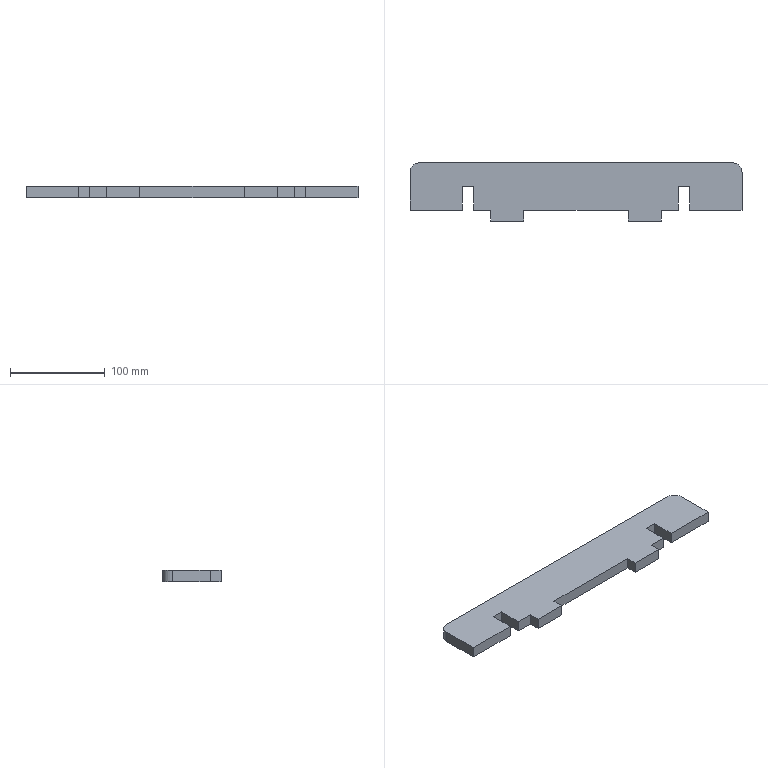Part | SolidWorks | features FlatPattern 1, SMBaseFlange 1, SheetMetal 1 | 1 solid | 24 faces | box 350 x 61.5 x 12 mm | volume 211887 mm3 | plane 22 | cylinder 2 | commonest cylinder face diameters 20 x2
STEP:
#1=CARTESIAN_POINT('',(212.445,-154.972,0.));
#2=VERTEX_POINT('',#1);
#3=CARTESIAN_POINT('',(212.445,-114.972,0.));
#4=VERTEX_POINT('',#3);
#5=CARTESIAN_POINT('',(212.445,-154.972,0.));
#6=DIRECTION('',(0.,1.,0.));
#7=VECTOR('',#6,1000.);
#8=LINE('',#5,#7);
#9=EDGE_CURVE('',#2,#4,#8,.T.);
#10=ORIENTED_EDGE('',*,*,#9,.F.);
#11=CARTESIAN_POINT('',(212.445,-154.972,-12.));
#12=VERTEX_POINT('',#11);
#13=CARTESIAN_POINT('',(212.445,-154.972,-12.));
#14=DIRECTION('',(0.,0.,1.));
#15=VECTOR('',#14,1000.);
#16=LINE('',#13,#15);
#17=EDGE_CURVE('',#12,#2,#16,.T.);
#18=ORIENTED_EDGE('',*,*,#17,.F.);
#19=CARTESIAN_POINT('',(212.445,-114.972,-12.));
#20=VERTEX_POINT('',#19);
#21=CARTESIAN_POINT('',(212.445,-154.972,-12.));
#22=DIRECTION('',(0.,1.,0.));
#23=VECTOR('',#22,1000.);
#24=LINE('',#21,#23);
#25=EDGE_CURVE('',#12,#20,#24,.T.);
#26=ORIENTED_EDGE('',*,*,#25,.T.);
#27=CARTESIAN_POINT('',(212.445,-114.972,-12.));
#28=DIRECTION('',(0.,0.,1.));
#29=VECTOR('',#28,1000.);
#30=LINE('',#27,#29);
#31=EDGE_CURVE('',#20,#4,#30,.T.);
#32=ORIENTED_EDGE('',*,*,#31,.T.);
#33=EDGE_LOOP('',(#10,#18,#26,#32));
#34=FACE_OUTER_BOUND('',#33,.T.);
#35=CARTESIAN_POINT('',(212.445,-154.972,-12.));
#36=DIRECTION('',(1.,0.,0.));
#37=DIRECTION('',(0.,0.,-1.));
#38=AXIS2_PLACEMENT_3D('',#35,#36,#37);
#39=PLANE('',#38);
#40=ADVANCED_FACE('',(#34),#39,.T.);
#41=CARTESIAN_POINT('',(157.445,-154.972,0.));
#42=VERTEX_POINT('',#41);
#43=CARTESIAN_POINT('',(212.445,-154.972,0.));
#44=DIRECTION('',(1.,0.,0.));
#45=VECTOR('',#44,1000.);
#46=LINE('',#43,#45);
#47=EDGE_CURVE('',#42,#2,#46,.T.);
#48=ORIENTED_EDGE('',*,*,#47,.F.);
#49=CARTESIAN_POINT('',(157.445,-154.972,-12.));
#50=VERTEX_POINT('',#49);
#51=CARTESIAN_POINT('',(157.445,-154.972,-12.));
#52=DIRECTION('',(0.,0.,1.));
#53=VECTOR('',#52,1000.);
#54=LINE('',#51,#53);
#55=EDGE_CURVE('',#50,#42,#54,.T.);
#56=ORIENTED_EDGE('',*,*,#55,.F.);
#57=CARTESIAN_POINT('',(212.445,-154.972,-12.));
#58=DIRECTION('',(1.,0.,0.));
#59=VECTOR('',#58,1000.);
#60=LINE('',#57,#59);
#61=EDGE_CURVE('',#50,#12,#60,.T.);
#62=ORIENTED_EDGE('',*,*,#61,.T.);
#63=ORIENTED_EDGE('',*,*,#17,.T.);
#64=EDGE_LOOP('',(#48,#56,#62,#63));
#65=FACE_OUTER_BOUND('',#64,.T.);
#66=CARTESIAN_POINT('',(212.445,-154.972,-12.));
#67=DIRECTION('',(0.,-1.,0.));
#68=DIRECTION('',(1.,0.,0.));
#69=AXIS2_PLACEMENT_3D('',#66,#67,#68);
#70=PLANE('',#69);
#71=ADVANCED_FACE('',(#65),#70,.T.);
#72=CARTESIAN_POINT('',(157.445,-129.772,0.));
#73=VERTEX_POINT('',#72);
#74=CARTESIAN_POINT('',(157.445,-129.772,0.));
#75=DIRECTION('',(0.,-1.,0.));
#76=VECTOR('',#75,1000.);
#77=LINE('',#74,#76);
#78=EDGE_CURVE('',#73,#42,#77,.T.);
#79=ORIENTED_EDGE('',*,*,#78,.F.);
#80=CARTESIAN_POINT('',(157.445,-129.772,-12.));
#81=VERTEX_POINT('',#80);
#82=CARTESIAN_POINT('',(157.445,-129.772,-12.));
#83=DIRECTION('',(0.,0.,1.));
#84=VECTOR('',#83,1000.);
#85=LINE('',#82,#84);
#86=EDGE_CURVE('',#81,#73,#85,.T.);
#87=ORIENTED_EDGE('',*,*,#86,.F.);
#88=CARTESIAN_POINT('',(157.445,-129.772,-12.));
#89=DIRECTION('',(0.,-1.,0.));
#90=VECTOR('',#89,1000.);
#91=LINE('',#88,#90);
#92=EDGE_CURVE('',#81,#50,#91,.T.);
#93=ORIENTED_EDGE('',*,*,#92,.T.);
#94=ORIENTED_EDGE('',*,*,#55,.T.);
#95=EDGE_LOOP('',(#79,#87,#93,#94));
#96=FACE_OUTER_BOUND('',#95,.T.);
#97=CARTESIAN_POINT('',(157.445,-129.772,-12.));
#98=DIRECTION('',(-1.,0.,0.));
#99=DIRECTION('',(0.,0.,1.));
#100=AXIS2_PLACEMENT_3D('',#97,#98,#99);
#101=PLANE('',#100);
#102=ADVANCED_FACE('',(#96),#101,.T.);
#103=CARTESIAN_POINT('',(145.445,-129.772,0.));
#104=VERTEX_POINT('',#103);
#105=CARTESIAN_POINT('',(145.445,-129.772,0.));
#106=DIRECTION('',(1.,0.,0.));
#107=VECTOR('',#106,1000.);
#108=LINE('',#105,#107);
#109=EDGE_CURVE('',#104,#73,#108,.T.);
#110=ORIENTED_EDGE('',*,*,#109,.F.);
#111=CARTESIAN_POINT('',(145.445,-129.772,-12.));
#112=VERTEX_POINT('',#111);
#113=CARTESIAN_POINT('',(145.445,-129.772,-12.));
#114=DIRECTION('',(0.,0.,1.));
#115=VECTOR('',#114,1000.);
#116=LINE('',#113,#115);
#117=EDGE_CURVE('',#112,#104,#116,.T.);
#118=ORIENTED_EDGE('',*,*,#117,.F.);
#119=CARTESIAN_POINT('',(145.445,-129.772,-12.));
#120=DIRECTION('',(1.,0.,0.));
#121=VECTOR('',#120,1000.);
#122=LINE('',#119,#121);
#123=EDGE_CURVE('',#112,#81,#122,.T.);
#124=ORIENTED_EDGE('',*,*,#123,.T.);
#125=ORIENTED_EDGE('',*,*,#86,.T.);
#126=EDGE_LOOP('',(#110,#118,#124,#125));
#127=FACE_OUTER_BOUND('',#126,.T.);
#128=CARTESIAN_POINT('',(145.445,-129.772,-12.));
#129=DIRECTION('',(0.,-1.,0.));
#130=DIRECTION('',(0.,0.,-1.));
#131=AXIS2_PLACEMENT_3D('',#128,#129,#130);
#132=PLANE('',#131);
#133=ADVANCED_FACE('',(#127),#132,.T.);
#134=CARTESIAN_POINT('',(145.445,-154.972,0.));
#135=VERTEX_POINT('',#134);
#136=CARTESIAN_POINT('',(145.445,-154.972,0.));
#137=DIRECTION('',(0.,1.,0.));
#138=VECTOR('',#137,1000.);
#139=LINE('',#136,#138);
#140=EDGE_CURVE('',#135,#104,#139,.T.);
#141=ORIENTED_EDGE('',*,*,#140,.F.);
#142=CARTESIAN_POINT('',(145.445,-154.972,-12.));
#143=VERTEX_POINT('',#142);
#144=CARTESIAN_POINT('',(145.445,-154.972,-12.));
#145=DIRECTION('',(0.,0.,1.));
#146=VECTOR('',#145,1000.);
#147=LINE('',#144,#146);
#148=EDGE_CURVE('',#143,#135,#147,.T.);
#149=ORIENTED_EDGE('',*,*,#148,.F.);
#150=CARTESIAN_POINT('',(145.445,-154.972,-12.));
#151=DIRECTION('',(0.,1.,0.));
#152=VECTOR('',#151,1000.);
#153=LINE('',#150,#152);
#154=EDGE_CURVE('',#143,#112,#153,.T.);
#155=ORIENTED_EDGE('',*,*,#154,.T.);
#156=ORIENTED_EDGE('',*,*,#117,.T.);
#157=EDGE_LOOP('',(#141,#149,#155,#156));
#158=FACE_OUTER_BOUND('',#157,.T.);
#159=CARTESIAN_POINT('',(145.445,-154.972,-12.));
#160=DIRECTION('',(1.,0.,0.));
#161=DIRECTION('',(0.,0.,-1.));
#162=AXIS2_PLACEMENT_3D('',#159,#160,#161);
#163=PLANE('',#162);
#164=ADVANCED_FACE('',(#158),#163,.T.);
#165=CARTESIAN_POINT('',(127.445,-154.972,0.));
#166=VERTEX_POINT('',#165);
#167=CARTESIAN_POINT('',(145.445,-154.972,0.));
#168=DIRECTION('',(1.,0.,0.));
#169=VECTOR('',#168,1000.);
#170=LINE('',#167,#169);
#171=EDGE_CURVE('',#166,#135,#170,.T.);
#172=ORIENTED_EDGE('',*,*,#171,.F.);
#173=CARTESIAN_POINT('',(127.445,-154.972,-12.));
#174=VERTEX_POINT('',#173);
#175=CARTESIAN_POINT('',(127.445,-154.972,-12.));
#176=DIRECTION('',(0.,0.,1.));
#177=VECTOR('',#176,1000.);
#178=LINE('',#175,#177);
#179=EDGE_CURVE('',#174,#166,#178,.T.);
#180=ORIENTED_EDGE('',*,*,#179,.F.);
#181=CARTESIAN_POINT('',(145.445,-154.972,-12.));
#182=DIRECTION('',(1.,0.,0.));
#183=VECTOR('',#182,1000.);
#184=LINE('',#181,#183);
#185=EDGE_CURVE('',#174,#143,#184,.T.);
#186=ORIENTED_EDGE('',*,*,#185,.T.);
#187=ORIENTED_EDGE('',*,*,#148,.T.);
#188=EDGE_LOOP('',(#172,#180,#186,#187));
#189=FACE_OUTER_BOUND('',#188,.T.);
#190=CARTESIAN_POINT('',(145.445,-154.972,-12.));
#191=DIRECTION('',(0.,-1.,0.));
#192=DIRECTION('',(1.,0.,0.));
#193=AXIS2_PLACEMENT_3D('',#190,#191,#192);
#194=PLANE('',#193);
#195=ADVANCED_FACE('',(#189),#194,.T.);
#196=CARTESIAN_POINT('',(127.445,-166.472,0.));
#197=VERTEX_POINT('',#196);
#198=CARTESIAN_POINT('',(127.445,-154.972,0.));
#199=DIRECTION('',(0.,1.,0.));
#200=VECTOR('',#199,1000.);
#201=LINE('',#198,#200);
#202=EDGE_CURVE('',#197,#166,#201,.T.);
#203=ORIENTED_EDGE('',*,*,#202,.F.);
#204=CARTESIAN_POINT('',(127.445,-166.472,-12.));
#205=VERTEX_POINT('',#204);
#206=CARTESIAN_POINT('',(127.445,-166.472,-12.));
#207=DIRECTION('',(0.,0.,1.));
#208=VECTOR('',#207,1000.);
#209=LINE('',#206,#208);
#210=EDGE_CURVE('',#205,#197,#209,.T.);
#211=ORIENTED_EDGE('',*,*,#210,.F.);
#212=CARTESIAN_POINT('',(127.445,-154.972,-12.));
#213=DIRECTION('',(0.,1.,0.));
#214=VECTOR('',#213,1000.);
#215=LINE('',#212,#214);
#216=EDGE_CURVE('',#205,#174,#215,.T.);
#217=ORIENTED_EDGE('',*,*,#216,.T.);
#218=ORIENTED_EDGE('',*,*,#179,.T.);
#219=EDGE_LOOP('',(#203,#211,#217,#218));
#220=FACE_OUTER_BOUND('',#219,.T.);
#221=CARTESIAN_POINT('',(127.445,-154.972,-12.));
#222=DIRECTION('',(1.,0.,0.));
#223=DIRECTION('',(0.,1.,0.));
#224=AXIS2_PLACEMENT_3D('',#221,#222,#223);
#225=PLANE('',#224);
#226=ADVANCED_FACE('',(#220),#225,.T.);
#227=CARTESIAN_POINT('',(92.445,-166.472,0.));
#228=VERTEX_POINT('',#227);
#229=CARTESIAN_POINT('',(127.445,-166.472,0.));
#230=DIRECTION('',(1.,0.,0.));
#231=VECTOR('',#230,1000.);
#232=LINE('',#229,#231);
#233=EDGE_CURVE('',#228,#197,#232,.T.);
#234=ORIENTED_EDGE('',*,*,#233,.F.);
#235=CARTESIAN_POINT('',(92.445,-166.472,-12.));
#236=VERTEX_POINT('',#235);
#237=CARTESIAN_POINT('',(92.445,-166.472,-12.));
#238=DIRECTION('',(0.,0.,1.));
#239=VECTOR('',#238,1000.);
#240=LINE('',#237,#239);
#241=EDGE_CURVE('',#236,#228,#240,.T.);
#242=ORIENTED_EDGE('',*,*,#241,.F.);
#243=CARTESIAN_POINT('',(127.445,-166.472,-12.));
#244=DIRECTION('',(1.,0.,0.));
#245=VECTOR('',#244,1000.);
#246=LINE('',#243,#245);
#247=EDGE_CURVE('',#236,#205,#246,.T.);
#248=ORIENTED_EDGE('',*,*,#247,.T.);
#249=ORIENTED_EDGE('',*,*,#210,.T.);
#250=EDGE_LOOP('',(#234,#242,#248,#249));
#251=FACE_OUTER_BOUND('',#250,.T.);
#252=CARTESIAN_POINT('',(127.445,-166.472,-12.));
#253=DIRECTION('',(0.,-1.,0.));
#254=DIRECTION('',(0.,0.,-1.));
#255=AXIS2_PLACEMENT_3D('',#252,#253,#254);
#256=PLANE('',#255);
#257=ADVANCED_FACE('',(#251),#256,.T.);
#258=CARTESIAN_POINT('',(92.445,-154.972,0.));
#259=VERTEX_POINT('',#258);
#260=CARTESIAN_POINT('',(92.445,-166.472,0.));
#261=DIRECTION('',(0.,-1.,0.));
#262=VECTOR('',#261,1000.);
#263=LINE('',#260,#262);
#264=EDGE_CURVE('',#259,#228,#263,.T.);
#265=ORIENTED_EDGE('',*,*,#264,.F.);
#266=CARTESIAN_POINT('',(92.445,-154.972,-12.));
#267=VERTEX_POINT('',#266);
#268=CARTESIAN_POINT('',(92.445,-154.972,-12.));
#269=DIRECTION('',(0.,0.,1.));
#270=VECTOR('',#269,1000.);
#271=LINE('',#268,#270);
#272=EDGE_CURVE('',#267,#259,#271,.T.);
#273=ORIENTED_EDGE('',*,*,#272,.F.);
#274=CARTESIAN_POINT('',(92.445,-166.472,-12.));
#275=DIRECTION('',(0.,-1.,0.));
#276=VECTOR('',#275,1000.);
#277=LINE('',#274,#276);
#278=EDGE_CURVE('',#267,#236,#277,.T.);
#279=ORIENTED_EDGE('',*,*,#278,.T.);
#280=ORIENTED_EDGE('',*,*,#241,.T.);
#281=EDGE_LOOP('',(#265,#273,#279,#280));
#282=FACE_OUTER_BOUND('',#281,.T.);
#283=CARTESIAN_POINT('',(92.445,-166.472,-12.));
#284=DIRECTION('',(-1.,0.,0.));
#285=DIRECTION('',(0.,0.,1.));
#286=AXIS2_PLACEMENT_3D('',#283,#284,#285);
#287=PLANE('',#286);
#288=ADVANCED_FACE('',(#282),#287,.T.);
#289=CARTESIAN_POINT('',(-17.555,-154.972,0.));
#290=VERTEX_POINT('',#289);
#291=CARTESIAN_POINT('',(92.445,-154.972,0.));
#292=DIRECTION('',(1.,0.,0.));
#293=VECTOR('',#292,1000.);
#294=LINE('',#291,#293);
#295=EDGE_CURVE('',#290,#259,#294,.T.);
#296=ORIENTED_EDGE('',*,*,#295,.F.);
#297=CARTESIAN_POINT('',(-17.555,-154.972,-12.));
#298=VERTEX_POINT('',#297);
#299=CARTESIAN_POINT('',(-17.555,-154.972,-12.));
#300=DIRECTION('',(0.,0.,1.));
#301=VECTOR('',#300,1000.);
#302=LINE('',#299,#301);
#303=EDGE_CURVE('',#298,#290,#302,.T.);
#304=ORIENTED_EDGE('',*,*,#303,.F.);
#305=CARTESIAN_POINT('',(92.445,-154.972,-12.));
#306=DIRECTION('',(1.,0.,0.));
#307=VECTOR('',#306,1000.);
#308=LINE('',#305,#307);
#309=EDGE_CURVE('',#298,#267,#308,.T.);
#310=ORIENTED_EDGE('',*,*,#309,.T.);
#311=ORIENTED_EDGE('',*,*,#272,.T.);
#312=EDGE_LOOP('',(#296,#304,#310,#311));
#313=FACE_OUTER_BOUND('',#312,.T.);
#314=CARTESIAN_POINT('',(92.445,-154.972,-12.));
#315=DIRECTION('',(0.,-1.,0.));
#316=DIRECTION('',(0.,0.,-1.));
#317=AXIS2_PLACEMENT_3D('',#314,#315,#316);
#318=PLANE('',#317);
#319=ADVANCED_FACE('',(#313),#318,.T.);
#320=CARTESIAN_POINT('',(-17.555,-166.472,0.));
#321=VERTEX_POINT('',#320);
#322=CARTESIAN_POINT('',(-17.555,-166.472,0.));
#323=DIRECTION('',(0.,1.,0.));
#324=VECTOR('',#323,1000.);
#325=LINE('',#322,#324);
#326=EDGE_CURVE('',#321,#290,#325,.T.);
#327=ORIENTED_EDGE('',*,*,#326,.F.);
#328=CARTESIAN_POINT('',(-17.555,-166.472,-12.));
#329=VERTEX_POINT('',#328);
#330=CARTESIAN_POINT('',(-17.555,-166.472,-12.));
#331=DIRECTION('',(0.,0.,1.));
#332=VECTOR('',#331,1000.);
#333=LINE('',#330,#332);
#334=EDGE_CURVE('',#329,#321,#333,.T.);
#335=ORIENTED_EDGE('',*,*,#334,.F.);
#336=CARTESIAN_POINT('',(-17.555,-166.472,-12.));
#337=DIRECTION('',(0.,1.,0.));
#338=VECTOR('',#337,1000.);
#339=LINE('',#336,#338);
#340=EDGE_CURVE('',#329,#298,#339,.T.);
#341=ORIENTED_EDGE('',*,*,#340,.T.);
#342=ORIENTED_EDGE('',*,*,#303,.T.);
#343=EDGE_LOOP('',(#327,#335,#341,#342));
#344=FACE_OUTER_BOUND('',#343,.T.);
#345=CARTESIAN_POINT('',(-17.555,-166.472,-12.));
#346=DIRECTION('',(1.,0.,0.));
#347=DIRECTION('',(0.,0.,-1.));
#348=AXIS2_PLACEMENT_3D('',#345,#346,#347);
#349=PLANE('',#348);
#350=ADVANCED_FACE('',(#344),#349,.T.);
#351=CARTESIAN_POINT('',(-52.555,-166.472,0.));
#352=VERTEX_POINT('',#351);
#353=CARTESIAN_POINT('',(-52.555,-166.472,0.));
#354=DIRECTION('',(1.,0.,0.));
#355=VECTOR('',#354,1000.);
#356=LINE('',#353,#355);
#357=EDGE_CURVE('',#352,#321,#356,.T.);
#358=ORIENTED_EDGE('',*,*,#357,.F.);
#359=CARTESIAN_POINT('',(-52.555,-166.472,-12.));
#360=VERTEX_POINT('',#359);
#361=CARTESIAN_POINT('',(-52.555,-166.472,-12.));
#362=DIRECTION('',(0.,0.,1.));
#363=VECTOR('',#362,1000.);
#364=LINE('',#361,#363);
#365=EDGE_CURVE('',#360,#352,#364,.T.);
#366=ORIENTED_EDGE('',*,*,#365,.F.);
#367=CARTESIAN_POINT('',(-52.555,-166.472,-12.));
#368=DIRECTION('',(1.,0.,0.));
#369=VECTOR('',#368,1000.);
#370=LINE('',#367,#369);
#371=EDGE_CURVE('',#360,#329,#370,.T.);
#372=ORIENTED_EDGE('',*,*,#371,.T.);
#373=ORIENTED_EDGE('',*,*,#334,.T.);
#374=EDGE_LOOP('',(#358,#366,#372,#373));
#375=FACE_OUTER_BOUND('',#374,.T.);
#376=CARTESIAN_POINT('',(-52.555,-166.472,-12.));
#377=DIRECTION('',(0.,-1.,0.));
#378=DIRECTION('',(0.,0.,-1.));
#379=AXIS2_PLACEMENT_3D('',#376,#377,#378);
#380=PLANE('',#379);
#381=ADVANCED_FACE('',(#375),#380,.T.);
#382=CARTESIAN_POINT('',(-52.555,-154.972,0.));
#383=VERTEX_POINT('',#382);
#384=CARTESIAN_POINT('',(-52.555,-154.972,0.));
#385=DIRECTION('',(0.,-1.,0.));
#386=VECTOR('',#385,1000.);
#387=LINE('',#384,#386);
#388=EDGE_CURVE('',#383,#352,#387,.T.);
#389=ORIENTED_EDGE('',*,*,#388,.F.);
#390=CARTESIAN_POINT('',(-52.555,-154.972,-12.));
#391=VERTEX_POINT('',#390);
#392=CARTESIAN_POINT('',(-52.555,-154.972,-12.));
#393=DIRECTION('',(0.,0.,1.));
#394=VECTOR('',#393,1000.);
#395=LINE('',#392,#394);
#396=EDGE_CURVE('',#391,#383,#395,.T.);
#397=ORIENTED_EDGE('',*,*,#396,.F.);
#398=CARTESIAN_POINT('',(-52.555,-154.972,-12.));
#399=DIRECTION('',(0.,-1.,0.));
#400=VECTOR('',#399,1000.);
#401=LINE('',#398,#400);
#402=EDGE_CURVE('',#391,#360,#401,.T.);
#403=ORIENTED_EDGE('',*,*,#402,.T.);
#404=ORIENTED_EDGE('',*,*,#365,.T.);
#405=EDGE_LOOP('',(#389,#397,#403,#404));
#406=FACE_OUTER_BOUND('',#405,.T.);
#407=CARTESIAN_POINT('',(-52.555,-154.972,-12.));
#408=DIRECTION('',(-1.,0.,0.));
#409=DIRECTION('',(0.,-1.,0.));
#410=AXIS2_PLACEMENT_3D('',#407,#408,#409);
#411=PLANE('',#410);
#412=ADVANCED_FACE('',(#406),#411,.T.);
#413=CARTESIAN_POINT('',(-70.555,-154.972,0.));
#414=VERTEX_POINT('',#413);
#415=CARTESIAN_POINT('',(-52.555,-154.972,0.));
#416=DIRECTION('',(1.,0.,0.));
#417=VECTOR('',#416,1000.);
#418=LINE('',#415,#417);
#419=EDGE_CURVE('',#414,#383,#418,.T.);
#420=ORIENTED_EDGE('',*,*,#419,.F.);
#421=CARTESIAN_POINT('',(-70.555,-154.972,-12.));
#422=VERTEX_POINT('',#421);
#423=CARTESIAN_POINT('',(-70.555,-154.972,-12.));
#424=DIRECTION('',(0.,0.,1.));
#425=VECTOR('',#424,1000.);
#426=LINE('',#423,#425);
#427=EDGE_CURVE('',#422,#414,#426,.T.);
#428=ORIENTED_EDGE('',*,*,#427,.F.);
#429=CARTESIAN_POINT('',(-52.555,-154.972,-12.));
#430=DIRECTION('',(1.,0.,0.));
#431=VECTOR('',#430,1000.);
#432=LINE('',#429,#431);
#433=EDGE_CURVE('',#422,#391,#432,.T.);
#434=ORIENTED_EDGE('',*,*,#433,.T.);
#435=ORIENTED_EDGE('',*,*,#396,.T.);
#436=EDGE_LOOP('',(#420,#428,#434,#435));
#437=FACE_OUTER_BOUND('',#436,.T.);
#438=CARTESIAN_POINT('',(-52.555,-154.972,-12.));
#439=DIRECTION('',(0.,-1.,0.));
#440=DIRECTION('',(1.,0.,0.));
#441=AXIS2_PLACEMENT_3D('',#438,#439,#440);
#442=PLANE('',#441);
#443=ADVANCED_FACE('',(#437),#442,.T.);
#444=CARTESIAN_POINT('',(-70.555,-129.772,0.));
#445=VERTEX_POINT('',#444);
#446=CARTESIAN_POINT('',(-70.555,-129.772,0.));
#447=DIRECTION('',(0.,-1.,0.));
#448=VECTOR('',#447,1000.);
#449=LINE('',#446,#448);
#450=EDGE_CURVE('',#445,#414,#449,.T.);
#451=ORIENTED_EDGE('',*,*,#450,.F.);
#452=CARTESIAN_POINT('',(-70.555,-129.772,-12.));
#453=VERTEX_POINT('',#452);
#454=CARTESIAN_POINT('',(-70.555,-129.772,-12.));
#455=DIRECTION('',(0.,0.,1.));
#456=VECTOR('',#455,1000.);
#457=LINE('',#454,#456);
#458=EDGE_CURVE('',#453,#445,#457,.T.);
#459=ORIENTED_EDGE('',*,*,#458,.F.);
#460=CARTESIAN_POINT('',(-70.555,-129.772,-12.));
#461=DIRECTION('',(0.,-1.,0.));
#462=VECTOR('',#461,1000.);
#463=LINE('',#460,#462);
#464=EDGE_CURVE('',#453,#422,#463,.T.);
#465=ORIENTED_EDGE('',*,*,#464,.T.);
#466=ORIENTED_EDGE('',*,*,#427,.T.);
#467=EDGE_LOOP('',(#451,#459,#465,#466));
#468=FACE_OUTER_BOUND('',#467,.T.);
#469=CARTESIAN_POINT('',(-70.555,-129.772,-12.));
#470=DIRECTION('',(-1.,0.,0.));
#471=DIRECTION('',(0.,0.,1.));
#472=AXIS2_PLACEMENT_3D('',#469,#470,#471);
#473=PLANE('',#472);
#474=ADVANCED_FACE('',(#468),#473,.T.);
#475=CARTESIAN_POINT('',(-82.555,-129.772,0.));
#476=VERTEX_POINT('',#475);
#477=CARTESIAN_POINT('',(-82.555,-129.772,0.));
#478=DIRECTION('',(1.,0.,0.));
#479=VECTOR('',#478,1000.);
#480=LINE('',#477,#479);
#481=EDGE_CURVE('',#476,#445,#480,.T.);
#482=ORIENTED_EDGE('',*,*,#481,.F.);
#483=CARTESIAN_POINT('',(-82.555,-129.772,-12.));
#484=VERTEX_POINT('',#483);
#485=CARTESIAN_POINT('',(-82.555,-129.772,-12.));
#486=DIRECTION('',(0.,0.,1.));
#487=VECTOR('',#486,1000.);
#488=LINE('',#485,#487);
#489=EDGE_CURVE('',#484,#476,#488,.T.);
#490=ORIENTED_EDGE('',*,*,#489,.F.);
#491=CARTESIAN_POINT('',(-82.555,-129.772,-12.));
#492=DIRECTION('',(1.,0.,0.));
#493=VECTOR('',#492,1000.);
#494=LINE('',#491,#493);
#495=EDGE_CURVE('',#484,#453,#494,.T.);
#496=ORIENTED_EDGE('',*,*,#495,.T.);
#497=ORIENTED_EDGE('',*,*,#458,.T.);
#498=EDGE_LOOP('',(#482,#490,#496,#497));
#499=FACE_OUTER_BOUND('',#498,.T.);
#500=CARTESIAN_POINT('',(-82.555,-129.772,-12.));
#501=DIRECTION('',(0.,-1.,0.));
#502=DIRECTION('',(0.,0.,-1.));
#503=AXIS2_PLACEMENT_3D('',#500,#501,#502);
#504=PLANE('',#503);
#505=ADVANCED_FACE('',(#499),#504,.T.);
#506=CARTESIAN_POINT('',(-82.555,-154.972,0.));
#507=VERTEX_POINT('',#506);
#508=CARTESIAN_POINT('',(-82.555,-154.972,0.));
#509=DIRECTION('',(0.,1.,0.));
#510=VECTOR('',#509,1000.);
#511=LINE('',#508,#510);
#512=EDGE_CURVE('',#507,#476,#511,.T.);
#513=ORIENTED_EDGE('',*,*,#512,.F.);
#514=CARTESIAN_POINT('',(-82.555,-154.972,-12.));
#515=VERTEX_POINT('',#514);
#516=CARTESIAN_POINT('',(-82.555,-154.972,-12.));
#517=DIRECTION('',(0.,0.,1.));
#518=VECTOR('',#517,1000.);
#519=LINE('',#516,#518);
#520=EDGE_CURVE('',#515,#507,#519,.T.);
#521=ORIENTED_EDGE('',*,*,#520,.F.);
#522=CARTESIAN_POINT('',(-82.555,-154.972,-12.));
#523=DIRECTION('',(0.,1.,0.));
#524=VECTOR('',#523,1000.);
#525=LINE('',#522,#524);
#526=EDGE_CURVE('',#515,#484,#525,.T.);
#527=ORIENTED_EDGE('',*,*,#526,.T.);
#528=ORIENTED_EDGE('',*,*,#489,.T.);
#529=EDGE_LOOP('',(#513,#521,#527,#528));
#530=FACE_OUTER_BOUND('',#529,.T.);
#531=CARTESIAN_POINT('',(-82.555,-154.972,-12.));
#532=DIRECTION('',(1.,0.,0.));
#533=DIRECTION('',(0.,0.,-1.));
#534=AXIS2_PLACEMENT_3D('',#531,#532,#533);
#535=PLANE('',#534);
#536=ADVANCED_FACE('',(#530),#535,.T.);
#537=CARTESIAN_POINT('',(-137.555,-154.972,0.));
#538=VERTEX_POINT('',#537);
#539=CARTESIAN_POINT('',(-82.555,-154.972,0.));
#540=DIRECTION('',(1.,0.,0.));
#541=VECTOR('',#540,1000.);
#542=LINE('',#539,#541);
#543=EDGE_CURVE('',#538,#507,#542,.T.);
#544=ORIENTED_EDGE('',*,*,#543,.F.);
#545=CARTESIAN_POINT('',(-137.555,-154.972,-12.));
#546=VERTEX_POINT('',#545);
#547=CARTESIAN_POINT('',(-137.555,-154.972,-12.));
#548=DIRECTION('',(0.,0.,1.));
#549=VECTOR('',#548,1000.);
#550=LINE('',#547,#549);
#551=EDGE_CURVE('',#546,#538,#550,.T.);
#552=ORIENTED_EDGE('',*,*,#551,.F.);
#553=CARTESIAN_POINT('',(-82.555,-154.972,-12.));
#554=DIRECTION('',(1.,0.,0.));
#555=VECTOR('',#554,1000.);
#556=LINE('',#553,#555);
#557=EDGE_CURVE('',#546,#515,#556,.T.);
#558=ORIENTED_EDGE('',*,*,#557,.T.);
#559=ORIENTED_EDGE('',*,*,#520,.T.);
#560=EDGE_LOOP('',(#544,#552,#558,#559));
#561=FACE_OUTER_BOUND('',#560,.T.);
#562=CARTESIAN_POINT('',(-82.555,-154.972,-12.));
#563=DIRECTION('',(0.,-1.,0.));
#564=DIRECTION('',(1.,0.,0.));
#565=AXIS2_PLACEMENT_3D('',#562,#563,#564);
#566=PLANE('',#565);
#567=ADVANCED_FACE('',(#561),#566,.T.);
#568=CARTESIAN_POINT('',(-137.555,-114.972,0.));
#569=VERTEX_POINT('',#568);
#570=CARTESIAN_POINT('',(-137.555,-154.972,0.));
#571=DIRECTION('',(0.,-1.,0.));
#572=VECTOR('',#571,1000.);
#573=LINE('',#570,#572);
#574=EDGE_CURVE('',#569,#538,#573,.T.);
#575=ORIENTED_EDGE('',*,*,#574,.F.);
#576=CARTESIAN_POINT('',(-137.555,-114.972,-12.));
#577=VERTEX_POINT('',#576);
#578=CARTESIAN_POINT('',(-137.555,-114.972,-12.));
#579=DIRECTION('',(0.,0.,1.));
#580=VECTOR('',#579,1000.);
#581=LINE('',#578,#580);
#582=EDGE_CURVE('',#577,#569,#581,.T.);
#583=ORIENTED_EDGE('',*,*,#582,.F.);
#584=CARTESIAN_POINT('',(-137.555,-154.972,-12.));
#585=DIRECTION('',(0.,-1.,0.));
#586=VECTOR('',#585,1000.);
#587=LINE('',#584,#586);
#588=EDGE_CURVE('',#577,#546,#587,.T.);
#589=ORIENTED_EDGE('',*,*,#588,.T.);
#590=ORIENTED_EDGE('',*,*,#551,.T.);
#591=EDGE_LOOP('',(#575,#583,#589,#590));
#592=FACE_OUTER_BOUND('',#591,.T.);
#593=CARTESIAN_POINT('',(-137.555,-154.972,-12.));
#594=DIRECTION('',(-1.,0.,0.));
#595=DIRECTION('',(0.,0.,1.));
#596=AXIS2_PLACEMENT_3D('',#593,#594,#595);
#597=PLANE('',#596);
#598=ADVANCED_FACE('',(#592),#597,.T.);
#599=CARTESIAN_POINT('',(-127.555,-104.972,0.));
#600=VERTEX_POINT('',#599);
#601=CARTESIAN_POINT('',(-127.555,-114.972,0.));
#602=DIRECTION('',(0.,0.,1.));
#603=DIRECTION('',(1.,0.,0.));
#604=AXIS2_PLACEMENT_3D('',#601,#602,#603);
#605=CIRCLE('',#604,10.);
#606=EDGE_CURVE('',#600,#569,#605,.T.);
#607=ORIENTED_EDGE('',*,*,#606,.F.);
#608=CARTESIAN_POINT('',(-127.555,-104.972,-12.));
#609=VERTEX_POINT('',#608);
#610=CARTESIAN_POINT('',(-127.555,-104.972,-12.));
#611=DIRECTION('',(0.,0.,1.));
#612=VECTOR('',#611,1000.);
#613=LINE('',#610,#612);
#614=EDGE_CURVE('',#609,#600,#613,.T.);
#615=ORIENTED_EDGE('',*,*,#614,.F.);
#616=CARTESIAN_POINT('',(-127.555,-114.972,-12.));
#617=DIRECTION('',(0.,0.,1.));
#618=DIRECTION('',(1.,0.,0.));
#619=AXIS2_PLACEMENT_3D('',#616,#617,#618);
#620=CIRCLE('',#619,10.);
#621=EDGE_CURVE('',#609,#577,#620,.T.);
#622=ORIENTED_EDGE('',*,*,#621,.T.);
#623=ORIENTED_EDGE('',*,*,#582,.T.);
#624=EDGE_LOOP('',(#607,#615,#622,#623));
#625=FACE_OUTER_BOUND('',#624,.T.);
#626=CARTESIAN_POINT('',(-127.555,-114.972,-12.));
#627=DIRECTION('',(0.,0.,1.));
#628=DIRECTION('',(1.,0.,0.));
#629=AXIS2_PLACEMENT_3D('',#626,#627,#628);
#630=CYLINDRICAL_SURFACE('',#629,10.);
#631=ADVANCED_FACE('',(#625),#630,.T.);
#632=CARTESIAN_POINT('',(202.445,-104.972,0.));
#633=VERTEX_POINT('',#632);
#634=CARTESIAN_POINT('',(202.445,-104.972,0.));
#635=DIRECTION('',(-1.,0.,0.));
#636=VECTOR('',#635,1000.);
#637=LINE('',#634,#636);
#638=EDGE_CURVE('',#633,#600,#637,.T.);
#639=ORIENTED_EDGE('',*,*,#638,.F.);
#640=CARTESIAN_POINT('',(202.445,-104.972,-12.));
#641=VERTEX_POINT('',#640);
#642=CARTESIAN_POINT('',(202.445,-104.972,-12.));
#643=DIRECTION('',(0.,0.,1.));
#644=VECTOR('',#643,1000.);
#645=LINE('',#642,#644);
#646=EDGE_CURVE('',#641,#633,#645,.T.);
#647=ORIENTED_EDGE('',*,*,#646,.F.);
#648=CARTESIAN_POINT('',(202.445,-104.972,-12.));
#649=DIRECTION('',(-1.,0.,0.));
#650=VECTOR('',#649,1000.);
#651=LINE('',#648,#650);
#652=EDGE_CURVE('',#641,#609,#651,.T.);
#653=ORIENTED_EDGE('',*,*,#652,.T.);
#654=ORIENTED_EDGE('',*,*,#614,.T.);
#655=EDGE_LOOP('',(#639,#647,#653,#654));
#656=FACE_OUTER_BOUND('',#655,.T.);
#657=CARTESIAN_POINT('',(202.445,-104.972,-12.));
#658=DIRECTION('',(0.,1.,0.));
#659=DIRECTION('',(-1.,0.,0.));
#660=AXIS2_PLACEMENT_3D('',#657,#658,#659);
#661=PLANE('',#660);
#662=ADVANCED_FACE('',(#656),#661,.T.);
#663=CARTESIAN_POINT('',(202.445,-114.972,0.));
#664=DIRECTION('',(0.,0.,1.));
#665=DIRECTION('',(1.,0.,0.));
#666=AXIS2_PLACEMENT_3D('',#663,#664,#665);
#667=CIRCLE('',#666,10.);
#668=EDGE_CURVE('',#4,#633,#667,.T.);
#669=ORIENTED_EDGE('',*,*,#668,.F.);
#670=ORIENTED_EDGE('',*,*,#31,.F.);
#671=CARTESIAN_POINT('',(202.445,-114.972,-12.));
#672=DIRECTION('',(0.,0.,1.));
#673=DIRECTION('',(1.,0.,0.));
#674=AXIS2_PLACEMENT_3D('',#671,#672,#673);
#675=CIRCLE('',#674,10.);
#676=EDGE_CURVE('',#20,#641,#675,.T.);
#677=ORIENTED_EDGE('',*,*,#676,.T.);
#678=ORIENTED_EDGE('',*,*,#646,.T.);
#679=EDGE_LOOP('',(#669,#670,#677,#678));
#680=FACE_OUTER_BOUND('',#679,.T.);
#681=CARTESIAN_POINT('',(202.445,-114.972,-12.));
#682=DIRECTION('',(0.,0.,1.));
#683=DIRECTION('',(1.,0.,0.));
#684=AXIS2_PLACEMENT_3D('',#681,#682,#683);
#685=CYLINDRICAL_SURFACE('',#684,10.);
#686=ADVANCED_FACE('',(#680),#685,.T.);
#687=ORIENTED_EDGE('',*,*,#25,.F.);
#688=ORIENTED_EDGE('',*,*,#61,.F.);
#689=ORIENTED_EDGE('',*,*,#92,.F.);
#690=ORIENTED_EDGE('',*,*,#123,.F.);
#691=ORIENTED_EDGE('',*,*,#154,.F.);
#692=ORIENTED_EDGE('',*,*,#185,.F.);
#693=ORIENTED_EDGE('',*,*,#216,.F.);
#694=ORIENTED_EDGE('',*,*,#247,.F.);
#695=ORIENTED_EDGE('',*,*,#278,.F.);
#696=ORIENTED_EDGE('',*,*,#309,.F.);
#697=ORIENTED_EDGE('',*,*,#340,.F.);
#698=ORIENTED_EDGE('',*,*,#371,.F.);
#699=ORIENTED_EDGE('',*,*,#402,.F.);
#700=ORIENTED_EDGE('',*,*,#433,.F.);
#701=ORIENTED_EDGE('',*,*,#464,.F.);
#702=ORIENTED_EDGE('',*,*,#495,.F.);
#703=ORIENTED_EDGE('',*,*,#526,.F.);
#704=ORIENTED_EDGE('',*,*,#557,.F.);
#705=ORIENTED_EDGE('',*,*,#588,.F.);
#706=ORIENTED_EDGE('',*,*,#621,.F.);
#707=ORIENTED_EDGE('',*,*,#652,.F.);
#708=ORIENTED_EDGE('',*,*,#676,.F.);
#709=EDGE_LOOP('',(#687,#688,#689,#690,#691,#692,#693,#694,#695,#696,#697,#698,#699,#700,#701,#702,#703,#704,#705,#706,#707,#708));
#710=FACE_OUTER_BOUND('',#709,.T.);
#711=CARTESIAN_POINT('',(202.445,-114.972,-12.));
#712=DIRECTION('',(0.,0.,1.));
#713=DIRECTION('',(1.,0.,0.));
#714=AXIS2_PLACEMENT_3D('',#711,#712,#713);
#715=PLANE('',#714);
#716=ADVANCED_FACE('',(#710),#715,.F.);
#717=ORIENTED_EDGE('',*,*,#9,.T.);
#718=ORIENTED_EDGE('',*,*,#668,.T.);
#719=ORIENTED_EDGE('',*,*,#638,.T.);
#720=ORIENTED_EDGE('',*,*,#606,.T.);
#721=ORIENTED_EDGE('',*,*,#574,.T.);
#722=ORIENTED_EDGE('',*,*,#543,.T.);
#723=ORIENTED_EDGE('',*,*,#512,.T.);
#724=ORIENTED_EDGE('',*,*,#481,.T.);
#725=ORIENTED_EDGE('',*,*,#450,.T.);
#726=ORIENTED_EDGE('',*,*,#419,.T.);
#727=ORIENTED_EDGE('',*,*,#388,.T.);
#728=ORIENTED_EDGE('',*,*,#357,.T.);
#729=ORIENTED_EDGE('',*,*,#326,.T.);
#730=ORIENTED_EDGE('',*,*,#295,.T.);
#731=ORIENTED_EDGE('',*,*,#264,.T.);
#732=ORIENTED_EDGE('',*,*,#233,.T.);
#733=ORIENTED_EDGE('',*,*,#202,.T.);
#734=ORIENTED_EDGE('',*,*,#171,.T.);
#735=ORIENTED_EDGE('',*,*,#140,.T.);
#736=ORIENTED_EDGE('',*,*,#109,.T.);
#737=ORIENTED_EDGE('',*,*,#78,.T.);
#738=ORIENTED_EDGE('',*,*,#47,.T.);
#739=EDGE_LOOP('',(#717,#718,#719,#720,#721,#722,#723,#724,#725,#726,#727,#728,#729,#730,#731,#732,#733,#734,#735,#736,#737,#738));
#740=FACE_OUTER_BOUND('',#739,.T.);
#741=CARTESIAN_POINT('',(202.445,-114.972,0.));
#742=DIRECTION('',(0.,0.,1.));
#743=DIRECTION('',(1.,0.,0.));
#744=AXIS2_PLACEMENT_3D('',#741,#742,#743);
#745=PLANE('',#744);
#746=ADVANCED_FACE('',(#740),#745,.T.);
#747=CLOSED_SHELL('',(#40,#71,#102,#133,#164,#195,#226,#257,#288,#319,#350,#381,#412,#443,#474,#505,#536,#567,#598,#631,#662,#686,#716,#746));
#748=MANIFOLD_SOLID_BREP('',#747);
#749=CARTESIAN_POINT('',(0.,0.,0.));
#750=DIRECTION('',(0.,0.,1.));
#751=DIRECTION('',(1.,0.,0.));
#752=AXIS2_PLACEMENT_3D('',#749,#750,#751);
#753=(LENGTH_UNIT()NAMED_UNIT(*)SI_UNIT(.MILLI.,.METRE.));
#754=UNCERTAINTY_MEASURE_WITH_UNIT(LENGTH_MEASURE(0.00001),#753,'','');
#755=(NAMED_UNIT(*)PLANE_ANGLE_UNIT()SI_UNIT($,.RADIAN.));
#756=(NAMED_UNIT(*)SI_UNIT($,.STERADIAN.)SOLID_ANGLE_UNIT());
#757=(GEOMETRIC_REPRESENTATION_CONTEXT(3)GLOBAL_UNCERTAINTY_ASSIGNED_CONTEXT((#754))GLOBAL_UNIT_ASSIGNED_CONTEXT((#753,#755,#756))REPRESENTATION_CONTEXT('',''));
#758=ADVANCED_BREP_SHAPE_REPRESENTATION('',(#748,#752),#757);